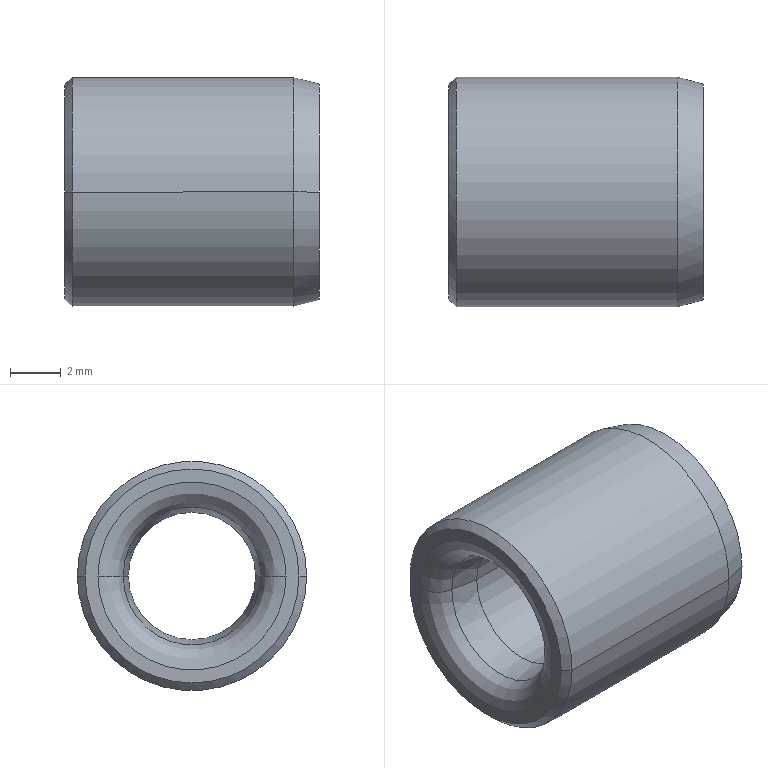Part | NX | 1 solid | 18 faces | box 10 x 9 x 9 mm | volume 417.945 mm3 | cone 8 | cylinder 4 | torus 4 | plane 2 | commonest cylinder face diameters 5 x2 9 x2
STEP:
#1=CARTESIAN_POINT('',(0.,-4.2,0.));
#2=VERTEX_POINT('',#1);
#3=CARTESIAN_POINT('',(0.,4.2,0.));
#4=VERTEX_POINT('',#3);
#5=CARTESIAN_POINT('',(0.,0.,0.));
#6=DIRECTION('',(-1.,0.,0.));
#7=DIRECTION('',(0.,1.,0.));
#8=AXIS2_PLACEMENT_3D('',#5,#6,#7);
#9=CIRCLE('',#8,4.2);
#10=EDGE_CURVE('',#2,#4,#9,.T.);
#11=ORIENTED_EDGE('',*,*,#10,.F.);
#12=CARTESIAN_POINT('',(0.3,-4.5,0.));
#13=VERTEX_POINT('',#12);
#14=CARTESIAN_POINT('',(0.15,-4.35,0.));
#15=DIRECTION('',(0.7071,-0.7071,0.));
#16=VECTOR('',#15,1000.);
#17=LINE('',#14,#16);
#18=EDGE_CURVE('',#13,#2,#17,.F.);
#19=ORIENTED_EDGE('',*,*,#18,.F.);
#20=CARTESIAN_POINT('',(0.3,4.5,0.));
#21=VERTEX_POINT('',#20);
#22=CARTESIAN_POINT('',(0.3,0.,0.));
#23=DIRECTION('',(-1.,0.,0.));
#24=DIRECTION('',(0.,1.,0.));
#25=AXIS2_PLACEMENT_3D('',#22,#23,#24);
#26=CIRCLE('',#25,4.5);
#27=EDGE_CURVE('',#13,#21,#26,.T.);
#28=ORIENTED_EDGE('',*,*,#27,.T.);
#29=CARTESIAN_POINT('',(0.15,4.35,0.));
#30=DIRECTION('',(0.7071,0.7071,0.));
#31=VECTOR('',#30,1000.);
#32=LINE('',#29,#31);
#33=EDGE_CURVE('',#21,#4,#32,.F.);
#34=ORIENTED_EDGE('',*,*,#33,.T.);
#35=EDGE_LOOP('',(#11,#19,#28,#34));
#36=FACE_BOUND('',#35,.T.);
#37=CARTESIAN_POINT('',(0.15,0.,0.));
#38=DIRECTION('',(1.,0.,0.));
#39=DIRECTION('',(0.,-1.,0.));
#40=AXIS2_PLACEMENT_3D('',#37,#38,#39);
#41=CONICAL_SURFACE('',#40,4.35,0.7854);
#42=ADVANCED_FACE('',(#36),#41,.T.);
#43=CARTESIAN_POINT('',(9.,4.5,0.));
#44=VERTEX_POINT('',#43);
#45=CARTESIAN_POINT('',(9.,-4.5,0.));
#46=VERTEX_POINT('',#45);
#47=CARTESIAN_POINT('',(9.,0.,0.));
#48=DIRECTION('',(-1.,0.,0.));
#49=DIRECTION('',(0.,1.,0.));
#50=AXIS2_PLACEMENT_3D('',#47,#48,#49);
#51=CIRCLE('',#50,4.5);
#52=EDGE_CURVE('',#44,#46,#51,.T.);
#53=ORIENTED_EDGE('',*,*,#52,.T.);
#54=CARTESIAN_POINT('',(4.65,-4.5,0.));
#55=DIRECTION('',(1.,0.,0.));
#56=VECTOR('',#55,1000.);
#57=LINE('',#54,#56);
#58=EDGE_CURVE('',#13,#46,#57,.T.);
#59=ORIENTED_EDGE('',*,*,#58,.F.);
#60=CARTESIAN_POINT('',(0.3,0.,0.));
#61=DIRECTION('',(-1.,0.,0.));
#62=DIRECTION('',(0.,1.,0.));
#63=AXIS2_PLACEMENT_3D('',#60,#61,#62);
#64=CIRCLE('',#63,4.5);
#65=EDGE_CURVE('',#21,#13,#64,.T.);
#66=ORIENTED_EDGE('',*,*,#65,.F.);
#67=CARTESIAN_POINT('',(4.65,4.5,0.));
#68=DIRECTION('',(1.,0.,0.));
#69=VECTOR('',#68,1000.);
#70=LINE('',#67,#69);
#71=EDGE_CURVE('',#21,#44,#70,.T.);
#72=ORIENTED_EDGE('',*,*,#71,.T.);
#73=EDGE_LOOP('',(#53,#59,#66,#72));
#74=FACE_BOUND('',#73,.T.);
#75=CARTESIAN_POINT('',(4.65,0.,0.));
#76=DIRECTION('',(1.,0.,0.));
#77=DIRECTION('',(0.,1.,0.));
#78=AXIS2_PLACEMENT_3D('',#75,#76,#77);
#79=CYLINDRICAL_SURFACE('',#78,4.5);
#80=ADVANCED_FACE('',(#74),#79,.T.);
#81=CARTESIAN_POINT('',(10.,4.232,0.));
#82=VERTEX_POINT('',#81);
#83=CARTESIAN_POINT('',(10.,-4.232,0.));
#84=VERTEX_POINT('',#83);
#85=CARTESIAN_POINT('',(10.,0.,0.));
#86=DIRECTION('',(-1.,0.,0.));
#87=DIRECTION('',(0.,1.,0.));
#88=AXIS2_PLACEMENT_3D('',#85,#86,#87);
#89=CIRCLE('',#88,4.232);
#90=EDGE_CURVE('',#82,#84,#89,.T.);
#91=ORIENTED_EDGE('',*,*,#90,.T.);
#92=CARTESIAN_POINT('',(9.5,-4.366,0.));
#93=DIRECTION('',(-0.9659,-0.2588,0.));
#94=VECTOR('',#93,1000.);
#95=LINE('',#92,#94);
#96=EDGE_CURVE('',#84,#46,#95,.T.);
#97=ORIENTED_EDGE('',*,*,#96,.T.);
#98=ORIENTED_EDGE('',*,*,#52,.F.);
#99=CARTESIAN_POINT('',(9.5,4.366,0.));
#100=DIRECTION('',(-0.9659,0.2588,0.));
#101=VECTOR('',#100,1000.);
#102=LINE('',#99,#101);
#103=EDGE_CURVE('',#82,#44,#102,.T.);
#104=ORIENTED_EDGE('',*,*,#103,.F.);
#105=EDGE_LOOP('',(#91,#97,#98,#104));
#106=FACE_BOUND('',#105,.T.);
#107=CARTESIAN_POINT('',(9.5,0.,0.));
#108=DIRECTION('',(-1.,0.,0.));
#109=DIRECTION('',(0.,1.,0.));
#110=AXIS2_PLACEMENT_3D('',#107,#108,#109);
#111=CONICAL_SURFACE('',#110,4.366,0.2618);
#112=ADVANCED_FACE('',(#106),#111,.T.);
#113=CARTESIAN_POINT('',(10.,-3.692,0.));
#114=VERTEX_POINT('',#113);
#115=CARTESIAN_POINT('',(10.,3.692,0.));
#116=VERTEX_POINT('',#115);
#117=CARTESIAN_POINT('',(10.,0.,0.));
#118=DIRECTION('',(-1.,0.,0.));
#119=DIRECTION('',(0.,1.,0.));
#120=AXIS2_PLACEMENT_3D('',#117,#118,#119);
#121=CIRCLE('',#120,3.692);
#122=EDGE_CURVE('',#114,#116,#121,.T.);
#123=ORIENTED_EDGE('',*,*,#122,.F.);
#124=CARTESIAN_POINT('',(9.174,-2.707,0.));
#125=VERTEX_POINT('',#124);
#126=CARTESIAN_POINT('',(9.,-3.692,0.));
#127=DIRECTION('',(0.,0.,1.));
#128=DIRECTION('',(-1.,0.,0.));
#129=AXIS2_PLACEMENT_3D('',#126,#127,#128);
#130=CIRCLE('',#129,1.);
#131=EDGE_CURVE('',#114,#125,#130,.T.);
#132=ORIENTED_EDGE('',*,*,#131,.T.);
#133=CARTESIAN_POINT('',(9.174,2.707,0.));
#134=VERTEX_POINT('',#133);
#135=CARTESIAN_POINT('',(9.174,0.,0.));
#136=DIRECTION('',(-1.,0.,0.));
#137=DIRECTION('',(0.,1.,0.));
#138=AXIS2_PLACEMENT_3D('',#135,#136,#137);
#139=CIRCLE('',#138,2.707);
#140=EDGE_CURVE('',#125,#134,#139,.T.);
#141=ORIENTED_EDGE('',*,*,#140,.T.);
#142=CARTESIAN_POINT('',(9.,3.692,0.));
#143=DIRECTION('',(0.,0.,-1.));
#144=DIRECTION('',(-1.,0.,0.));
#145=AXIS2_PLACEMENT_3D('',#142,#143,#144);
#146=CIRCLE('',#145,1.);
#147=EDGE_CURVE('',#116,#134,#146,.T.);
#148=ORIENTED_EDGE('',*,*,#147,.F.);
#149=EDGE_LOOP('',(#123,#132,#141,#148));
#150=FACE_BOUND('',#149,.T.);
#151=CARTESIAN_POINT('',(9.,0.,0.));
#152=DIRECTION('',(-1.,0.,0.));
#153=DIRECTION('',(0.,1.,0.));
#154=AXIS2_PLACEMENT_3D('',#151,#152,#153);
#155=TOROIDAL_SURFACE('',#154,3.692,1.);
#156=ADVANCED_FACE('',(#150),#155,.T.);
#157=ORIENTED_EDGE('',*,*,#140,.F.);
#158=CARTESIAN_POINT('',(8.,-2.5,0.));
#159=VERTEX_POINT('',#158);
#160=CARTESIAN_POINT('',(8.587,-2.603,0.));
#161=DIRECTION('',(0.9848,-0.1736,0.));
#162=VECTOR('',#161,1000.);
#163=LINE('',#160,#162);
#164=EDGE_CURVE('',#125,#159,#163,.F.);
#165=ORIENTED_EDGE('',*,*,#164,.T.);
#166=CARTESIAN_POINT('',(8.,2.5,0.));
#167=VERTEX_POINT('',#166);
#168=CARTESIAN_POINT('',(8.,0.,0.));
#169=DIRECTION('',(-1.,0.,0.));
#170=DIRECTION('',(0.,1.,0.));
#171=AXIS2_PLACEMENT_3D('',#168,#169,#170);
#172=CIRCLE('',#171,2.5);
#173=EDGE_CURVE('',#159,#167,#172,.T.);
#174=ORIENTED_EDGE('',*,*,#173,.T.);
#175=CARTESIAN_POINT('',(8.587,2.603,0.));
#176=DIRECTION('',(0.9848,0.1736,0.));
#177=VECTOR('',#176,1000.);
#178=LINE('',#175,#177);
#179=EDGE_CURVE('',#134,#167,#178,.F.);
#180=ORIENTED_EDGE('',*,*,#179,.F.);
#181=EDGE_LOOP('',(#157,#165,#174,#180));
#182=FACE_BOUND('',#181,.T.);
#183=CARTESIAN_POINT('',(8.587,0.,0.));
#184=DIRECTION('',(1.,0.,0.));
#185=DIRECTION('',(0.,-1.,0.));
#186=AXIS2_PLACEMENT_3D('',#183,#184,#185);
#187=CONICAL_SURFACE('',#186,2.603,0.1745);
#188=ADVANCED_FACE('',(#182),#187,.F.);
#189=CARTESIAN_POINT('',(2.,2.5,0.));
#190=VERTEX_POINT('',#189);
#191=CARTESIAN_POINT('',(2.,-2.5,0.));
#192=VERTEX_POINT('',#191);
#193=CARTESIAN_POINT('',(2.,0.,0.));
#194=DIRECTION('',(-1.,0.,0.));
#195=DIRECTION('',(0.,1.,0.));
#196=AXIS2_PLACEMENT_3D('',#193,#194,#195);
#197=CIRCLE('',#196,2.5);
#198=EDGE_CURVE('',#190,#192,#197,.T.);
#199=ORIENTED_EDGE('',*,*,#198,.T.);
#200=CARTESIAN_POINT('',(5.,-2.5,0.));
#201=DIRECTION('',(1.,0.,0.));
#202=VECTOR('',#201,1000.);
#203=LINE('',#200,#202);
#204=EDGE_CURVE('',#192,#159,#203,.T.);
#205=ORIENTED_EDGE('',*,*,#204,.T.);
#206=CARTESIAN_POINT('',(8.,0.,0.));
#207=DIRECTION('',(-1.,0.,0.));
#208=DIRECTION('',(0.,1.,0.));
#209=AXIS2_PLACEMENT_3D('',#206,#207,#208);
#210=CIRCLE('',#209,2.5);
#211=EDGE_CURVE('',#167,#159,#210,.T.);
#212=ORIENTED_EDGE('',*,*,#211,.F.);
#213=CARTESIAN_POINT('',(5.,2.5,0.));
#214=DIRECTION('',(1.,0.,0.));
#215=VECTOR('',#214,1000.);
#216=LINE('',#213,#215);
#217=EDGE_CURVE('',#190,#167,#216,.T.);
#218=ORIENTED_EDGE('',*,*,#217,.F.);
#219=EDGE_LOOP('',(#199,#205,#212,#218));
#220=FACE_BOUND('',#219,.T.);
#221=CARTESIAN_POINT('',(5.,0.,0.));
#222=DIRECTION('',(1.,0.,0.));
#223=DIRECTION('',(0.,1.,0.));
#224=AXIS2_PLACEMENT_3D('',#221,#222,#223);
#225=CYLINDRICAL_SURFACE('',#224,2.5);
#226=ADVANCED_FACE('',(#220),#225,.F.);
#227=CARTESIAN_POINT('',(0.8264,-2.707,0.));
#228=VERTEX_POINT('',#227);
#229=CARTESIAN_POINT('',(0.8264,2.707,0.));
#230=VERTEX_POINT('',#229);
#231=CARTESIAN_POINT('',(0.8264,0.,0.));
#232=DIRECTION('',(-1.,0.,0.));
#233=DIRECTION('',(0.,1.,0.));
#234=AXIS2_PLACEMENT_3D('',#231,#232,#233);
#235=CIRCLE('',#234,2.707);
#236=EDGE_CURVE('',#228,#230,#235,.T.);
#237=ORIENTED_EDGE('',*,*,#236,.T.);
#238=CARTESIAN_POINT('',(1.413,2.603,0.));
#239=DIRECTION('',(-0.9848,0.1736,0.));
#240=VECTOR('',#239,1000.);
#241=LINE('',#238,#240);
#242=EDGE_CURVE('',#190,#230,#241,.T.);
#243=ORIENTED_EDGE('',*,*,#242,.F.);
#244=CARTESIAN_POINT('',(2.,0.,0.));
#245=DIRECTION('',(-1.,0.,0.));
#246=DIRECTION('',(0.,1.,0.));
#247=AXIS2_PLACEMENT_3D('',#244,#245,#246);
#248=CIRCLE('',#247,2.5);
#249=EDGE_CURVE('',#192,#190,#248,.T.);
#250=ORIENTED_EDGE('',*,*,#249,.F.);
#251=CARTESIAN_POINT('',(1.413,-2.603,0.));
#252=DIRECTION('',(-0.9848,-0.1736,0.));
#253=VECTOR('',#252,1000.);
#254=LINE('',#251,#253);
#255=EDGE_CURVE('',#192,#228,#254,.T.);
#256=ORIENTED_EDGE('',*,*,#255,.T.);
#257=EDGE_LOOP('',(#237,#243,#250,#256));
#258=FACE_BOUND('',#257,.T.);
#259=CARTESIAN_POINT('',(1.413,0.,0.));
#260=DIRECTION('',(-1.,0.,0.));
#261=DIRECTION('',(0.,1.,0.));
#262=AXIS2_PLACEMENT_3D('',#259,#260,#261);
#263=CONICAL_SURFACE('',#262,2.603,0.1745);
#264=ADVANCED_FACE('',(#258),#263,.F.);
#265=ORIENTED_EDGE('',*,*,#236,.F.);
#266=CARTESIAN_POINT('',(0.,-3.692,0.));
#267=VERTEX_POINT('',#266);
#268=CARTESIAN_POINT('',(1.,-3.692,0.));
#269=DIRECTION('',(0.,0.,1.));
#270=DIRECTION('',(-1.,0.,0.));
#271=AXIS2_PLACEMENT_3D('',#268,#269,#270);
#272=CIRCLE('',#271,1.);
#273=EDGE_CURVE('',#267,#228,#272,.F.);
#274=ORIENTED_EDGE('',*,*,#273,.F.);
#275=CARTESIAN_POINT('',(0.,3.692,0.));
#276=VERTEX_POINT('',#275);
#277=CARTESIAN_POINT('',(0.,0.,0.));
#278=DIRECTION('',(-1.,0.,0.));
#279=DIRECTION('',(0.,1.,0.));
#280=AXIS2_PLACEMENT_3D('',#277,#278,#279);
#281=CIRCLE('',#280,3.692);
#282=EDGE_CURVE('',#267,#276,#281,.T.);
#283=ORIENTED_EDGE('',*,*,#282,.T.);
#284=CARTESIAN_POINT('',(1.,3.692,0.));
#285=DIRECTION('',(0.,0.,-1.));
#286=DIRECTION('',(-1.,0.,0.));
#287=AXIS2_PLACEMENT_3D('',#284,#285,#286);
#288=CIRCLE('',#287,1.);
#289=EDGE_CURVE('',#276,#230,#288,.F.);
#290=ORIENTED_EDGE('',*,*,#289,.T.);
#291=EDGE_LOOP('',(#265,#274,#283,#290));
#292=FACE_BOUND('',#291,.T.);
#293=CARTESIAN_POINT('',(1.,0.,0.));
#294=DIRECTION('',(-1.,0.,0.));
#295=DIRECTION('',(0.,1.,0.));
#296=AXIS2_PLACEMENT_3D('',#293,#294,#295);
#297=TOROIDAL_SURFACE('',#296,3.692,1.);
#298=ADVANCED_FACE('',(#292),#297,.T.);
#299=ORIENTED_EDGE('',*,*,#10,.T.);
#300=CARTESIAN_POINT('',(0.,0.,0.));
#301=DIRECTION('',(-1.,0.,0.));
#302=DIRECTION('',(0.,1.,0.));
#303=AXIS2_PLACEMENT_3D('',#300,#301,#302);
#304=CIRCLE('',#303,4.2);
#305=EDGE_CURVE('',#4,#2,#304,.T.);
#306=ORIENTED_EDGE('',*,*,#305,.T.);
#307=EDGE_LOOP('',(#299,#306));
#308=FACE_BOUND('',#307,.T.);
#309=CARTESIAN_POINT('',(0.,0.,0.));
#310=DIRECTION('',(-1.,0.,0.));
#311=DIRECTION('',(0.,1.,0.));
#312=AXIS2_PLACEMENT_3D('',#309,#310,#311);
#313=CIRCLE('',#312,3.692);
#314=EDGE_CURVE('',#276,#267,#313,.T.);
#315=ORIENTED_EDGE('',*,*,#314,.F.);
#316=ORIENTED_EDGE('',*,*,#282,.F.);
#317=EDGE_LOOP('',(#315,#316));
#318=FACE_BOUND('',#317,.T.);
#319=CARTESIAN_POINT('',(0.,3.946,0.));
#320=DIRECTION('',(-1.,0.,0.));
#321=DIRECTION('',(0.,0.,1.));
#322=AXIS2_PLACEMENT_3D('',#319,#320,#321);
#323=PLANE('',#322);
#324=ADVANCED_FACE('',(#308,#318),#323,.T.);
#325=ORIENTED_EDGE('',*,*,#90,.F.);
#326=CARTESIAN_POINT('',(10.,0.,0.));
#327=DIRECTION('',(-1.,0.,0.));
#328=DIRECTION('',(0.,1.,0.));
#329=AXIS2_PLACEMENT_3D('',#326,#327,#328);
#330=CIRCLE('',#329,4.232);
#331=EDGE_CURVE('',#84,#82,#330,.T.);
#332=ORIENTED_EDGE('',*,*,#331,.F.);
#333=EDGE_LOOP('',(#325,#332));
#334=FACE_BOUND('',#333,.T.);
#335=ORIENTED_EDGE('',*,*,#122,.T.);
#336=CARTESIAN_POINT('',(10.,0.,0.));
#337=DIRECTION('',(-1.,0.,0.));
#338=DIRECTION('',(0.,1.,0.));
#339=AXIS2_PLACEMENT_3D('',#336,#337,#338);
#340=CIRCLE('',#339,3.692);
#341=EDGE_CURVE('',#116,#114,#340,.T.);
#342=ORIENTED_EDGE('',*,*,#341,.T.);
#343=EDGE_LOOP('',(#335,#342));
#344=FACE_BOUND('',#343,.T.);
#345=CARTESIAN_POINT('',(10.,3.962,0.));
#346=DIRECTION('',(1.,0.,0.));
#347=DIRECTION('',(0.,-1.,0.));
#348=AXIS2_PLACEMENT_3D('',#345,#346,#347);
#349=PLANE('',#348);
#350=ADVANCED_FACE('',(#334,#344),#349,.T.);
#351=ORIENTED_EDGE('',*,*,#211,.T.);
#352=ORIENTED_EDGE('',*,*,#164,.F.);
#353=CARTESIAN_POINT('',(9.174,0.,0.));
#354=DIRECTION('',(-1.,0.,0.));
#355=DIRECTION('',(0.,1.,0.));
#356=AXIS2_PLACEMENT_3D('',#353,#354,#355);
#357=CIRCLE('',#356,2.707);
#358=EDGE_CURVE('',#134,#125,#357,.T.);
#359=ORIENTED_EDGE('',*,*,#358,.F.);
#360=ORIENTED_EDGE('',*,*,#179,.T.);
#361=EDGE_LOOP('',(#351,#352,#359,#360));
#362=FACE_BOUND('',#361,.T.);
#363=CARTESIAN_POINT('',(8.587,0.,0.));
#364=DIRECTION('',(1.,0.,0.));
#365=DIRECTION('',(0.,-1.,0.));
#366=AXIS2_PLACEMENT_3D('',#363,#364,#365);
#367=CONICAL_SURFACE('',#366,2.603,0.1745);
#368=ADVANCED_FACE('',(#362),#367,.F.);
#369=ORIENTED_EDGE('',*,*,#217,.T.);
#370=ORIENTED_EDGE('',*,*,#173,.F.);
#371=ORIENTED_EDGE('',*,*,#204,.F.);
#372=ORIENTED_EDGE('',*,*,#249,.T.);
#373=EDGE_LOOP('',(#369,#370,#371,#372));
#374=FACE_BOUND('',#373,.T.);
#375=CARTESIAN_POINT('',(5.,0.,0.));
#376=DIRECTION('',(1.,0.,0.));
#377=DIRECTION('',(0.,1.,0.));
#378=AXIS2_PLACEMENT_3D('',#375,#376,#377);
#379=CYLINDRICAL_SURFACE('',#378,2.5);
#380=ADVANCED_FACE('',(#374),#379,.F.);
#381=ORIENTED_EDGE('',*,*,#198,.F.);
#382=ORIENTED_EDGE('',*,*,#242,.T.);
#383=CARTESIAN_POINT('',(0.8264,0.,0.));
#384=DIRECTION('',(-1.,0.,0.));
#385=DIRECTION('',(0.,1.,0.));
#386=AXIS2_PLACEMENT_3D('',#383,#384,#385);
#387=CIRCLE('',#386,2.707);
#388=EDGE_CURVE('',#230,#228,#387,.T.);
#389=ORIENTED_EDGE('',*,*,#388,.T.);
#390=ORIENTED_EDGE('',*,*,#255,.F.);
#391=EDGE_LOOP('',(#381,#382,#389,#390));
#392=FACE_BOUND('',#391,.T.);
#393=CARTESIAN_POINT('',(1.413,0.,0.));
#394=DIRECTION('',(-1.,0.,0.));
#395=DIRECTION('',(0.,1.,0.));
#396=AXIS2_PLACEMENT_3D('',#393,#394,#395);
#397=CONICAL_SURFACE('',#396,2.603,0.1745);
#398=ADVANCED_FACE('',(#392),#397,.F.);
#399=ORIENTED_EDGE('',*,*,#71,.F.);
#400=ORIENTED_EDGE('',*,*,#27,.F.);
#401=ORIENTED_EDGE('',*,*,#58,.T.);
#402=CARTESIAN_POINT('',(9.,0.,0.));
#403=DIRECTION('',(-1.,0.,0.));
#404=DIRECTION('',(0.,1.,0.));
#405=AXIS2_PLACEMENT_3D('',#402,#403,#404);
#406=CIRCLE('',#405,4.5);
#407=EDGE_CURVE('',#46,#44,#406,.T.);
#408=ORIENTED_EDGE('',*,*,#407,.T.);
#409=EDGE_LOOP('',(#399,#400,#401,#408));
#410=FACE_BOUND('',#409,.T.);
#411=CARTESIAN_POINT('',(4.65,0.,0.));
#412=DIRECTION('',(1.,0.,0.));
#413=DIRECTION('',(0.,1.,0.));
#414=AXIS2_PLACEMENT_3D('',#411,#412,#413);
#415=CYLINDRICAL_SURFACE('',#414,4.5);
#416=ADVANCED_FACE('',(#410),#415,.T.);
#417=ORIENTED_EDGE('',*,*,#103,.T.);
#418=ORIENTED_EDGE('',*,*,#407,.F.);
#419=ORIENTED_EDGE('',*,*,#96,.F.);
#420=ORIENTED_EDGE('',*,*,#331,.T.);
#421=EDGE_LOOP('',(#417,#418,#419,#420));
#422=FACE_BOUND('',#421,.T.);
#423=CARTESIAN_POINT('',(9.5,0.,0.));
#424=DIRECTION('',(-1.,0.,0.));
#425=DIRECTION('',(0.,1.,0.));
#426=AXIS2_PLACEMENT_3D('',#423,#424,#425);
#427=CONICAL_SURFACE('',#426,4.366,0.2618);
#428=ADVANCED_FACE('',(#422),#427,.T.);
#429=ORIENTED_EDGE('',*,*,#65,.T.);
#430=ORIENTED_EDGE('',*,*,#18,.T.);
#431=ORIENTED_EDGE('',*,*,#305,.F.);
#432=ORIENTED_EDGE('',*,*,#33,.F.);
#433=EDGE_LOOP('',(#429,#430,#431,#432));
#434=FACE_BOUND('',#433,.T.);
#435=CARTESIAN_POINT('',(0.15,0.,0.));
#436=DIRECTION('',(1.,0.,0.));
#437=DIRECTION('',(0.,-1.,0.));
#438=AXIS2_PLACEMENT_3D('',#435,#436,#437);
#439=CONICAL_SURFACE('',#438,4.35,0.7854);
#440=ADVANCED_FACE('',(#434),#439,.T.);
#441=ORIENTED_EDGE('',*,*,#147,.T.);
#442=ORIENTED_EDGE('',*,*,#358,.T.);
#443=ORIENTED_EDGE('',*,*,#131,.F.);
#444=ORIENTED_EDGE('',*,*,#341,.F.);
#445=EDGE_LOOP('',(#441,#442,#443,#444));
#446=FACE_BOUND('',#445,.T.);
#447=CARTESIAN_POINT('',(9.,0.,0.));
#448=DIRECTION('',(-1.,0.,0.));
#449=DIRECTION('',(0.,1.,0.));
#450=AXIS2_PLACEMENT_3D('',#447,#448,#449);
#451=TOROIDAL_SURFACE('',#450,3.692,1.);
#452=ADVANCED_FACE('',(#446),#451,.T.);
#453=ORIENTED_EDGE('',*,*,#314,.T.);
#454=ORIENTED_EDGE('',*,*,#273,.T.);
#455=ORIENTED_EDGE('',*,*,#388,.F.);
#456=ORIENTED_EDGE('',*,*,#289,.F.);
#457=EDGE_LOOP('',(#453,#454,#455,#456));
#458=FACE_BOUND('',#457,.T.);
#459=CARTESIAN_POINT('',(1.,0.,0.));
#460=DIRECTION('',(-1.,0.,0.));
#461=DIRECTION('',(0.,1.,0.));
#462=AXIS2_PLACEMENT_3D('',#459,#460,#461);
#463=TOROIDAL_SURFACE('',#462,3.692,1.);
#464=ADVANCED_FACE('',(#458),#463,.T.);
#465=CLOSED_SHELL('',(#42,#80,#112,#156,#188,#226,#264,#298,#324,#350,#368,#380,#398,#416,#428,#440,#452,#464));
#466=MANIFOLD_SOLID_BREP('',#465);
#467=(LENGTH_UNIT()NAMED_UNIT(*)SI_UNIT(.MILLI.,.METRE.));
#468=UNCERTAINTY_MEASURE_WITH_UNIT(LENGTH_MEASURE(0.00001),#467,'','');
#469=(NAMED_UNIT(*)PLANE_ANGLE_UNIT()SI_UNIT($,.RADIAN.));
#470=(NAMED_UNIT(*)SI_UNIT($,.STERADIAN.)SOLID_ANGLE_UNIT());
#471=(GEOMETRIC_REPRESENTATION_CONTEXT(3)GLOBAL_UNCERTAINTY_ASSIGNED_CONTEXT((#468))GLOBAL_UNIT_ASSIGNED_CONTEXT((#467,#469,#470))REPRESENTATION_CONTEXT('',''));
#472=ADVANCED_BREP_SHAPE_REPRESENTATION('',(#466),#471);